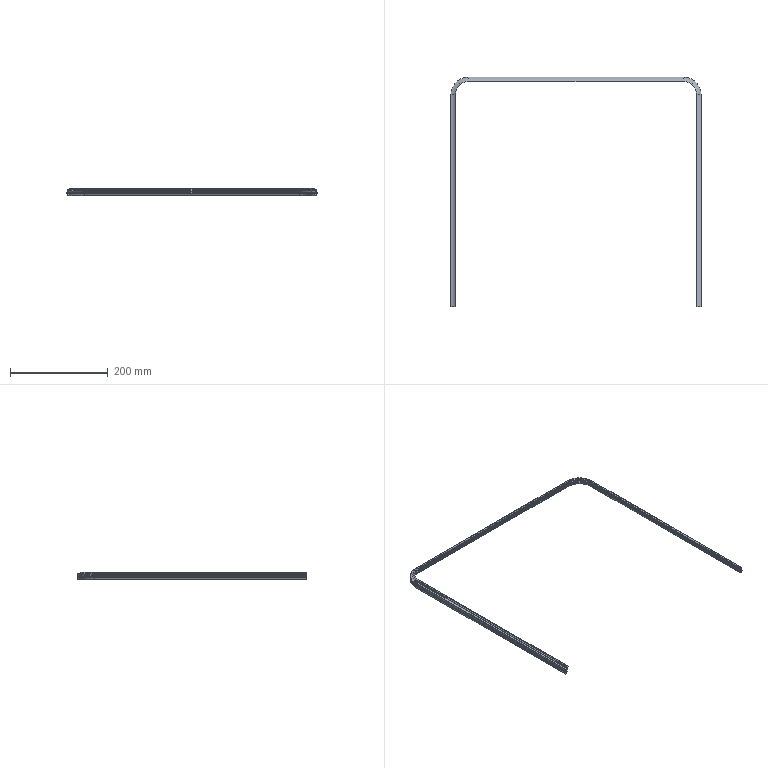Part | STEP file | ZXW722-L-35 | 1 solid | 188 faces | box 512.387 x 470.393 x 16.268 mm | volume 64395 mm3 | plane 66 | cylinder 54 | cone 36 | torus 32 | commonest cylinder face diameters 0.4 x15 0.2 x9 0.6 x9 1 x6 0.5 x3 38 x3